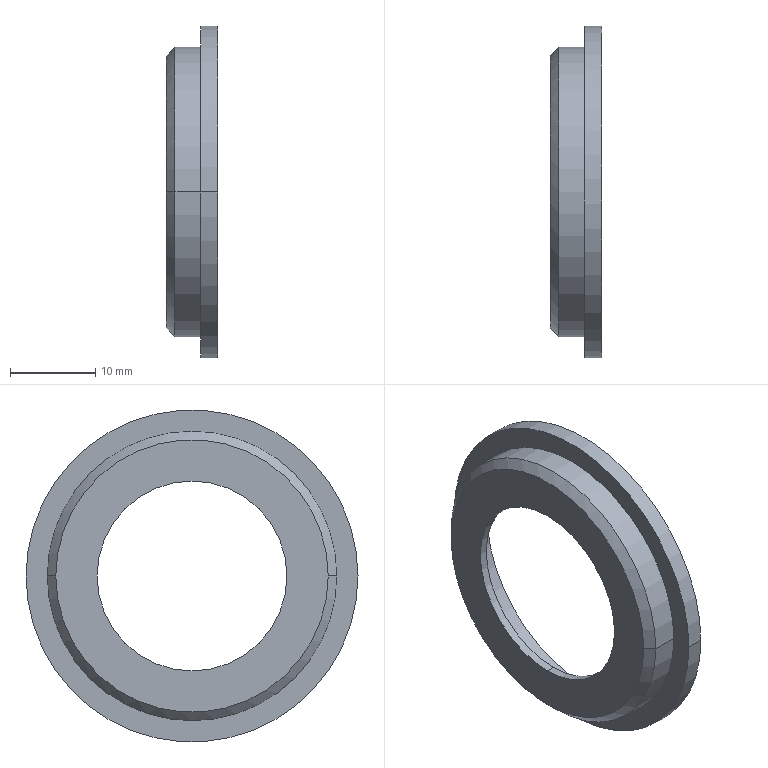Part | STEP file | Adjusting plate SGN-4-13 (19.5) | 1 solid | 15 faces | box 6 x 39 x 39 mm | volume 1841 mm3 | cylinder 8 | cone 4 | plane 3 | commonest cylinder face diameters 22.3 x2 32 x2 34 x2 39 x2
STEP:
#1=CARTESIAN_POINT('',(0.,0.,0.));
#2=DIRECTION('',(0.,0.,1.));
#3=DIRECTION('',(1.,0.,0.));
#4=AXIS2_PLACEMENT_3D('',#1,#2,#3);
#5=CARTESIAN_POINT('',(-6.,-16.,0.));
#6=VERTEX_POINT('',#5);
#7=CARTESIAN_POINT('',(-6.,16.,0.));
#8=VERTEX_POINT('',#7);
#9=CARTESIAN_POINT('',(-6.,0.,0.));
#10=DIRECTION('',(-1.,0.,0.));
#11=DIRECTION('',(0.,-1.,0.));
#12=AXIS2_PLACEMENT_3D('',#9,#10,#11);
#13=CIRCLE('',#12,16.);
#14=CARTESIAN_POINT('',(-5.,0.,0.));
#15=DIRECTION('',(1.,0.,0.));
#16=DIRECTION('',(0.,1.,0.));
#17=AXIS2_PLACEMENT_3D('',#14,#15,#16);
#18=CONICAL_SURFACE('',#17,17.,0.7854);
#19=CARTESIAN_POINT('',(3.142,-1.));
#20=DIRECTION('',(-1.,0.));
#21=VECTOR('',#20,1.);
#22=LINE('',#19,#21);
#23=(GEOMETRIC_REPRESENTATION_CONTEXT(2)PARAMETRIC_REPRESENTATION_CONTEXT()REPRESENTATION_CONTEXT('',''));
#24=DEFINITIONAL_REPRESENTATION('',(#22),#23);
#25=PCURVE('',#18,#24);
#26=CARTESIAN_POINT('',(-6.,17.,0.));
#27=DIRECTION('',(-1.,0.,0.));
#28=DIRECTION('',(0.,-1.,0.));
#29=AXIS2_PLACEMENT_3D('',#26,#27,#28);
#30=PLANE('',#29);
#31=CARTESIAN_POINT('',(17.,0.));
#32=DIRECTION('',(1.,0.));
#33=AXIS2_PLACEMENT_2D('',#31,#32);
#34=CIRCLE('',#33,16.);
#35=(GEOMETRIC_REPRESENTATION_CONTEXT(2)PARAMETRIC_REPRESENTATION_CONTEXT()REPRESENTATION_CONTEXT('',''));
#36=DEFINITIONAL_REPRESENTATION('',(#34),#35);
#37=PCURVE('',#30,#36);
#38=SURFACE_CURVE('',#13,(#25,#37),.PCURVE_S1.);
#39=EDGE_CURVE('',#6,#8,#38,.T.);
#40=ORIENTED_EDGE('',*,*,#39,.F.);
#41=CARTESIAN_POINT('',(-5.,-17.,0.));
#42=VERTEX_POINT('',#41);
#43=CARTESIAN_POINT('',(-5.,-17.,0.));
#44=DIRECTION('',(0.7071,-0.7071,0.));
#45=VECTOR('',#44,1.);
#46=LINE('',#43,#45);
#47=CARTESIAN_POINT('',(3.142,0.));
#48=DIRECTION('',(0.,1.));
#49=VECTOR('',#48,1.);
#50=LINE('',#47,#49);
#51=(GEOMETRIC_REPRESENTATION_CONTEXT(2)PARAMETRIC_REPRESENTATION_CONTEXT()REPRESENTATION_CONTEXT('',''));
#52=DEFINITIONAL_REPRESENTATION('',(#50),#51);
#53=PCURVE('',#18,#52);
#54=CARTESIAN_POINT('',(-5.,0.,0.));
#55=DIRECTION('',(1.,0.,0.));
#56=DIRECTION('',(0.,1.,0.));
#57=AXIS2_PLACEMENT_3D('',#54,#55,#56);
#58=CONICAL_SURFACE('',#57,17.,0.7854);
#59=CARTESIAN_POINT('',(3.142,0.));
#60=DIRECTION('',(0.,1.));
#61=VECTOR('',#60,1.);
#62=LINE('',#59,#61);
#63=(GEOMETRIC_REPRESENTATION_CONTEXT(2)PARAMETRIC_REPRESENTATION_CONTEXT()REPRESENTATION_CONTEXT('',''));
#64=DEFINITIONAL_REPRESENTATION('',(#62),#63);
#65=PCURVE('',#58,#64);
#66=SURFACE_CURVE('',#46,(#53,#65),.PCURVE_S1.);
#67=EDGE_CURVE('',#6,#42,#66,.T.);
#68=ORIENTED_EDGE('',*,*,#67,.T.);
#69=CARTESIAN_POINT('',(-5.,17.,0.));
#70=VERTEX_POINT('',#69);
#71=CARTESIAN_POINT('',(-5.,0.,0.));
#72=DIRECTION('',(1.,0.,0.));
#73=DIRECTION('',(0.,-1.,0.));
#74=AXIS2_PLACEMENT_3D('',#71,#72,#73);
#75=CIRCLE('',#74,17.);
#76=CARTESIAN_POINT('',(-3.142,0.));
#77=DIRECTION('',(1.,0.));
#78=VECTOR('',#77,1.);
#79=LINE('',#76,#78);
#80=(GEOMETRIC_REPRESENTATION_CONTEXT(2)PARAMETRIC_REPRESENTATION_CONTEXT()REPRESENTATION_CONTEXT('',''));
#81=DEFINITIONAL_REPRESENTATION('',(#79),#80);
#82=PCURVE('',#18,#81);
#83=CARTESIAN_POINT('',(0.,0.,0.));
#84=DIRECTION('',(1.,0.,0.));
#85=DIRECTION('',(0.,1.,0.));
#86=AXIS2_PLACEMENT_3D('',#83,#84,#85);
#87=CYLINDRICAL_SURFACE('',#86,17.);
#88=CARTESIAN_POINT('',(-3.142,-5.));
#89=DIRECTION('',(1.,0.));
#90=VECTOR('',#89,1.);
#91=LINE('',#88,#90);
#92=(GEOMETRIC_REPRESENTATION_CONTEXT(2)PARAMETRIC_REPRESENTATION_CONTEXT()REPRESENTATION_CONTEXT('',''));
#93=DEFINITIONAL_REPRESENTATION('',(#91),#92);
#94=PCURVE('',#87,#93);
#95=SURFACE_CURVE('',#75,(#82,#94),.PCURVE_S1.);
#96=EDGE_CURVE('',#70,#42,#95,.T.);
#97=ORIENTED_EDGE('',*,*,#96,.F.);
#98=CARTESIAN_POINT('',(-5.,17.,0.));
#99=DIRECTION('',(0.7071,0.7071,0.));
#100=VECTOR('',#99,1.);
#101=LINE('',#98,#100);
#102=CARTESIAN_POINT('',(0.,0.));
#103=DIRECTION('',(0.,1.));
#104=VECTOR('',#103,1.);
#105=LINE('',#102,#104);
#106=(GEOMETRIC_REPRESENTATION_CONTEXT(2)PARAMETRIC_REPRESENTATION_CONTEXT()REPRESENTATION_CONTEXT('',''));
#107=DEFINITIONAL_REPRESENTATION('',(#105),#106);
#108=PCURVE('',#18,#107);
#109=CARTESIAN_POINT('',(6.283,0.));
#110=DIRECTION('',(0.,1.));
#111=VECTOR('',#110,1.);
#112=LINE('',#109,#111);
#113=(GEOMETRIC_REPRESENTATION_CONTEXT(2)PARAMETRIC_REPRESENTATION_CONTEXT()REPRESENTATION_CONTEXT('',''));
#114=DEFINITIONAL_REPRESENTATION('',(#112),#113);
#115=PCURVE('',#58,#114);
#116=SURFACE_CURVE('',#101,(#108,#115),.PCURVE_S1.);
#117=EDGE_CURVE('',#8,#70,#116,.T.);
#118=ORIENTED_EDGE('',*,*,#117,.F.);
#119=EDGE_LOOP('',(#40,#68,#97,#118));
#120=FACE_BOUND('',#119,.T.);
#121=ADVANCED_FACE('',(#120),#18,.T.);
#122=CARTESIAN_POINT('',(-3.7,0.,-16.));
#123=VERTEX_POINT('',#122);
#124=CARTESIAN_POINT('',(0.,0.,-16.));
#125=VERTEX_POINT('',#124);
#126=CARTESIAN_POINT('',(0.,0.,-16.));
#127=DIRECTION('',(1.,0.,0.));
#128=VECTOR('',#127,1.);
#129=LINE('',#126,#128);
#130=CARTESIAN_POINT('',(0.,0.,0.));
#131=DIRECTION('',(1.,0.,0.));
#132=DIRECTION('',(0.,0.,-1.));
#133=AXIS2_PLACEMENT_3D('',#130,#131,#132);
#134=CYLINDRICAL_SURFACE('',#133,16.);
#135=CARTESIAN_POINT('',(6.283,0.));
#136=DIRECTION('',(0.,1.));
#137=VECTOR('',#136,1.);
#138=LINE('',#135,#137);
#139=(GEOMETRIC_REPRESENTATION_CONTEXT(2)PARAMETRIC_REPRESENTATION_CONTEXT()REPRESENTATION_CONTEXT('',''));
#140=DEFINITIONAL_REPRESENTATION('',(#138),#139);
#141=PCURVE('',#134,#140);
#142=CARTESIAN_POINT('',(0.,0.,0.));
#143=DIRECTION('',(1.,0.,0.));
#144=DIRECTION('',(0.,0.,-1.));
#145=AXIS2_PLACEMENT_3D('',#142,#143,#144);
#146=CYLINDRICAL_SURFACE('',#145,16.);
#147=CARTESIAN_POINT('',(0.,0.));
#148=DIRECTION('',(0.,1.));
#149=VECTOR('',#148,1.);
#150=LINE('',#147,#149);
#151=(GEOMETRIC_REPRESENTATION_CONTEXT(2)PARAMETRIC_REPRESENTATION_CONTEXT()REPRESENTATION_CONTEXT('',''));
#152=DEFINITIONAL_REPRESENTATION('',(#150),#151);
#153=PCURVE('',#146,#152);
#154=SURFACE_CURVE('',#129,(#141,#153),.PCURVE_S1.);
#155=EDGE_CURVE('',#123,#125,#154,.T.);
#156=ORIENTED_EDGE('',*,*,#155,.T.);
#157=CARTESIAN_POINT('',(0.,0.,16.));
#158=VERTEX_POINT('',#157);
#159=CARTESIAN_POINT('',(0.,0.,0.));
#160=DIRECTION('',(1.,0.,0.));
#161=DIRECTION('',(0.,0.,-1.));
#162=AXIS2_PLACEMENT_3D('',#159,#160,#161);
#163=CIRCLE('',#162,16.);
#164=CARTESIAN_POINT('',(0.,0.));
#165=DIRECTION('',(1.,0.));
#166=VECTOR('',#165,1.);
#167=LINE('',#164,#166);
#168=(GEOMETRIC_REPRESENTATION_CONTEXT(2)PARAMETRIC_REPRESENTATION_CONTEXT()REPRESENTATION_CONTEXT('',''));
#169=DEFINITIONAL_REPRESENTATION('',(#167),#168);
#170=PCURVE('',#134,#169);
#171=CARTESIAN_POINT('',(0.,0.,0.));
#172=DIRECTION('',(1.,0.,0.));
#173=DIRECTION('',(0.,1.,0.));
#174=AXIS2_PLACEMENT_3D('',#171,#172,#173);
#175=PLANE('',#174);
#176=CARTESIAN_POINT('',(0.,0.));
#177=DIRECTION('',(0.,-1.));
#178=AXIS2_PLACEMENT_2D('',#176,#177);
#179=CIRCLE('',#178,16.);
#180=(GEOMETRIC_REPRESENTATION_CONTEXT(2)PARAMETRIC_REPRESENTATION_CONTEXT()REPRESENTATION_CONTEXT('',''));
#181=DEFINITIONAL_REPRESENTATION('',(#179),#180);
#182=PCURVE('',#175,#181);
#183=SURFACE_CURVE('',#163,(#170,#182),.PCURVE_S1.);
#184=EDGE_CURVE('',#158,#125,#183,.T.);
#185=ORIENTED_EDGE('',*,*,#184,.F.);
#186=CARTESIAN_POINT('',(-3.7,0.,16.));
#187=VERTEX_POINT('',#186);
#188=CARTESIAN_POINT('',(0.,0.,16.));
#189=DIRECTION('',(1.,0.,0.));
#190=VECTOR('',#189,1.);
#191=LINE('',#188,#190);
#192=CARTESIAN_POINT('',(3.142,0.));
#193=DIRECTION('',(0.,1.));
#194=VECTOR('',#193,1.);
#195=LINE('',#192,#194);
#196=(GEOMETRIC_REPRESENTATION_CONTEXT(2)PARAMETRIC_REPRESENTATION_CONTEXT()REPRESENTATION_CONTEXT('',''));
#197=DEFINITIONAL_REPRESENTATION('',(#195),#196);
#198=PCURVE('',#134,#197);
#199=CARTESIAN_POINT('',(3.142,0.));
#200=DIRECTION('',(0.,1.));
#201=VECTOR('',#200,1.);
#202=LINE('',#199,#201);
#203=(GEOMETRIC_REPRESENTATION_CONTEXT(2)PARAMETRIC_REPRESENTATION_CONTEXT()REPRESENTATION_CONTEXT('',''));
#204=DEFINITIONAL_REPRESENTATION('',(#202),#203);
#205=PCURVE('',#146,#204);
#206=SURFACE_CURVE('',#191,(#198,#205),.PCURVE_S1.);
#207=EDGE_CURVE('',#187,#158,#206,.T.);
#208=ORIENTED_EDGE('',*,*,#207,.F.);
#209=CARTESIAN_POINT('',(-3.7,0.,0.));
#210=DIRECTION('',(1.,0.,0.));
#211=DIRECTION('',(0.,0.,-1.));
#212=AXIS2_PLACEMENT_3D('',#209,#210,#211);
#213=CIRCLE('',#212,16.);
#214=CARTESIAN_POINT('',(0.,-3.7));
#215=DIRECTION('',(1.,0.));
#216=VECTOR('',#215,1.);
#217=LINE('',#214,#216);
#218=(GEOMETRIC_REPRESENTATION_CONTEXT(2)PARAMETRIC_REPRESENTATION_CONTEXT()REPRESENTATION_CONTEXT('',''));
#219=DEFINITIONAL_REPRESENTATION('',(#217),#218);
#220=PCURVE('',#134,#219);
#221=CARTESIAN_POINT('',(-3.7,0.,0.));
#222=DIRECTION('',(1.,0.,0.));
#223=DIRECTION('',(0.,0.,-1.));
#224=AXIS2_PLACEMENT_3D('',#221,#222,#223);
#225=CONICAL_SURFACE('',#224,16.,1.309);
#226=CARTESIAN_POINT('',(0.,0.));
#227=DIRECTION('',(1.,0.));
#228=VECTOR('',#227,1.);
#229=LINE('',#226,#228);
#230=(GEOMETRIC_REPRESENTATION_CONTEXT(2)PARAMETRIC_REPRESENTATION_CONTEXT()REPRESENTATION_CONTEXT('',''));
#231=DEFINITIONAL_REPRESENTATION('',(#229),#230);
#232=PCURVE('',#225,#231);
#233=SURFACE_CURVE('',#213,(#220,#232),.PCURVE_S1.);
#234=EDGE_CURVE('',#187,#123,#233,.T.);
#235=ORIENTED_EDGE('',*,*,#234,.T.);
#236=EDGE_LOOP('',(#156,#185,#208,#235));
#237=FACE_BOUND('',#236,.F.);
#238=ADVANCED_FACE('',(#237),#134,.F.);
#239=CARTESIAN_POINT('',(-5.,0.,-11.15));
#240=VERTEX_POINT('',#239);
#241=CARTESIAN_POINT('',(-3.7,0.,-16.));
#242=DIRECTION('',(0.2588,0.,-0.9659));
#243=VECTOR('',#242,1.);
#244=LINE('',#241,#243);
#245=CARTESIAN_POINT('',(6.283,0.));
#246=DIRECTION('',(0.,1.));
#247=VECTOR('',#246,1.);
#248=LINE('',#245,#247);
#249=(GEOMETRIC_REPRESENTATION_CONTEXT(2)PARAMETRIC_REPRESENTATION_CONTEXT()REPRESENTATION_CONTEXT('',''));
#250=DEFINITIONAL_REPRESENTATION('',(#248),#249);
#251=PCURVE('',#225,#250);
#252=CARTESIAN_POINT('',(-3.7,0.,0.));
#253=DIRECTION('',(1.,0.,0.));
#254=DIRECTION('',(0.,0.,-1.));
#255=AXIS2_PLACEMENT_3D('',#252,#253,#254);
#256=CONICAL_SURFACE('',#255,16.,1.309);
#257=CARTESIAN_POINT('',(0.,0.));
#258=DIRECTION('',(0.,1.));
#259=VECTOR('',#258,1.);
#260=LINE('',#257,#259);
#261=(GEOMETRIC_REPRESENTATION_CONTEXT(2)PARAMETRIC_REPRESENTATION_CONTEXT()REPRESENTATION_CONTEXT('',''));
#262=DEFINITIONAL_REPRESENTATION('',(#260),#261);
#263=PCURVE('',#256,#262);
#264=SURFACE_CURVE('',#244,(#251,#263),.PCURVE_S1.);
#265=EDGE_CURVE('',#240,#123,#264,.T.);
#266=ORIENTED_EDGE('',*,*,#265,.T.);
#267=ORIENTED_EDGE('',*,*,#234,.F.);
#268=CARTESIAN_POINT('',(-5.,0.,11.15));
#269=VERTEX_POINT('',#268);
#270=CARTESIAN_POINT('',(-3.7,0.,16.));
#271=DIRECTION('',(0.2588,0.,0.9659));
#272=VECTOR('',#271,1.);
#273=LINE('',#270,#272);
#274=CARTESIAN_POINT('',(3.142,0.));
#275=DIRECTION('',(0.,1.));
#276=VECTOR('',#275,1.);
#277=LINE('',#274,#276);
#278=(GEOMETRIC_REPRESENTATION_CONTEXT(2)PARAMETRIC_REPRESENTATION_CONTEXT()REPRESENTATION_CONTEXT('',''));
#279=DEFINITIONAL_REPRESENTATION('',(#277),#278);
#280=PCURVE('',#225,#279);
#281=CARTESIAN_POINT('',(3.142,0.));
#282=DIRECTION('',(0.,1.));
#283=VECTOR('',#282,1.);
#284=LINE('',#281,#283);
#285=(GEOMETRIC_REPRESENTATION_CONTEXT(2)PARAMETRIC_REPRESENTATION_CONTEXT()REPRESENTATION_CONTEXT('',''));
#286=DEFINITIONAL_REPRESENTATION('',(#284),#285);
#287=PCURVE('',#256,#286);
#288=SURFACE_CURVE('',#273,(#280,#287),.PCURVE_S1.);
#289=EDGE_CURVE('',#269,#187,#288,.T.);
#290=ORIENTED_EDGE('',*,*,#289,.F.);
#291=CARTESIAN_POINT('',(-5.,0.,0.));
#292=DIRECTION('',(1.,0.,0.));
#293=DIRECTION('',(0.,0.,-1.));
#294=AXIS2_PLACEMENT_3D('',#291,#292,#293);
#295=CIRCLE('',#294,11.15);
#296=CARTESIAN_POINT('',(0.,-1.3));
#297=DIRECTION('',(1.,0.));
#298=VECTOR('',#297,1.);
#299=LINE('',#296,#298);
#300=(GEOMETRIC_REPRESENTATION_CONTEXT(2)PARAMETRIC_REPRESENTATION_CONTEXT()REPRESENTATION_CONTEXT('',''));
#301=DEFINITIONAL_REPRESENTATION('',(#299),#300);
#302=PCURVE('',#225,#301);
#303=CARTESIAN_POINT('',(-10.,0.,0.));
#304=DIRECTION('',(1.,0.,0.));
#305=DIRECTION('',(0.,0.,-1.));
#306=AXIS2_PLACEMENT_3D('',#303,#304,#305);
#307=CYLINDRICAL_SURFACE('',#306,11.15);
#308=CARTESIAN_POINT('',(0.,5.));
#309=DIRECTION('',(1.,0.));
#310=VECTOR('',#309,1.);
#311=LINE('',#308,#310);
#312=(GEOMETRIC_REPRESENTATION_CONTEXT(2)PARAMETRIC_REPRESENTATION_CONTEXT()REPRESENTATION_CONTEXT('',''));
#313=DEFINITIONAL_REPRESENTATION('',(#311),#312);
#314=PCURVE('',#307,#313);
#315=SURFACE_CURVE('',#295,(#302,#314),.PCURVE_S1.);
#316=EDGE_CURVE('',#269,#240,#315,.T.);
#317=ORIENTED_EDGE('',*,*,#316,.T.);
#318=EDGE_LOOP('',(#266,#267,#290,#317));
#319=FACE_BOUND('',#318,.F.);
#320=ADVANCED_FACE('',(#319),#225,.F.);
#321=CARTESIAN_POINT('',(-6.,0.,-11.15));
#322=VERTEX_POINT('',#321);
#323=CARTESIAN_POINT('',(-10.,0.,-11.15));
#324=DIRECTION('',(1.,0.,0.));
#325=VECTOR('',#324,1.);
#326=LINE('',#323,#325);
#327=CARTESIAN_POINT('',(6.283,0.));
#328=DIRECTION('',(0.,1.));
#329=VECTOR('',#328,1.);
#330=LINE('',#327,#329);
#331=(GEOMETRIC_REPRESENTATION_CONTEXT(2)PARAMETRIC_REPRESENTATION_CONTEXT()REPRESENTATION_CONTEXT('',''));
#332=DEFINITIONAL_REPRESENTATION('',(#330),#331);
#333=PCURVE('',#307,#332);
#334=CARTESIAN_POINT('',(-10.,0.,0.));
#335=DIRECTION('',(1.,0.,0.));
#336=DIRECTION('',(0.,0.,-1.));
#337=AXIS2_PLACEMENT_3D('',#334,#335,#336);
#338=CYLINDRICAL_SURFACE('',#337,11.15);
#339=CARTESIAN_POINT('',(0.,0.));
#340=DIRECTION('',(0.,1.));
#341=VECTOR('',#340,1.);
#342=LINE('',#339,#341);
#343=(GEOMETRIC_REPRESENTATION_CONTEXT(2)PARAMETRIC_REPRESENTATION_CONTEXT()REPRESENTATION_CONTEXT('',''));
#344=DEFINITIONAL_REPRESENTATION('',(#342),#343);
#345=PCURVE('',#338,#344);
#346=SURFACE_CURVE('',#326,(#333,#345),.PCURVE_S1.);
#347=EDGE_CURVE('',#322,#240,#346,.T.);
#348=ORIENTED_EDGE('',*,*,#347,.T.);
#349=ORIENTED_EDGE('',*,*,#316,.F.);
#350=CARTESIAN_POINT('',(-6.,0.,11.15));
#351=VERTEX_POINT('',#350);
#352=CARTESIAN_POINT('',(-10.,0.,11.15));
#353=DIRECTION('',(1.,0.,0.));
#354=VECTOR('',#353,1.);
#355=LINE('',#352,#354);
#356=CARTESIAN_POINT('',(3.142,0.));
#357=DIRECTION('',(0.,1.));
#358=VECTOR('',#357,1.);
#359=LINE('',#356,#358);
#360=(GEOMETRIC_REPRESENTATION_CONTEXT(2)PARAMETRIC_REPRESENTATION_CONTEXT()REPRESENTATION_CONTEXT('',''));
#361=DEFINITIONAL_REPRESENTATION('',(#359),#360);
#362=PCURVE('',#307,#361);
#363=CARTESIAN_POINT('',(3.142,0.));
#364=DIRECTION('',(0.,1.));
#365=VECTOR('',#364,1.);
#366=LINE('',#363,#365);
#367=(GEOMETRIC_REPRESENTATION_CONTEXT(2)PARAMETRIC_REPRESENTATION_CONTEXT()REPRESENTATION_CONTEXT('',''));
#368=DEFINITIONAL_REPRESENTATION('',(#366),#367);
#369=PCURVE('',#338,#368);
#370=SURFACE_CURVE('',#355,(#362,#369),.PCURVE_S1.);
#371=EDGE_CURVE('',#351,#269,#370,.T.);
#372=ORIENTED_EDGE('',*,*,#371,.F.);
#373=CARTESIAN_POINT('',(-6.,0.,0.));
#374=DIRECTION('',(-1.,0.,0.));
#375=DIRECTION('',(0.,-1.,0.));
#376=AXIS2_PLACEMENT_3D('',#373,#374,#375);
#377=CIRCLE('',#376,11.15);
#378=CARTESIAN_POINT('',(10.996,4.));
#379=DIRECTION('',(-1.,0.));
#380=VECTOR('',#379,1.);
#381=LINE('',#378,#380);
#382=(GEOMETRIC_REPRESENTATION_CONTEXT(2)PARAMETRIC_REPRESENTATION_CONTEXT()REPRESENTATION_CONTEXT('',''));
#383=DEFINITIONAL_REPRESENTATION('',(#381),#382);
#384=PCURVE('',#307,#383);
#385=CARTESIAN_POINT('',(17.,0.));
#386=DIRECTION('',(1.,0.));
#387=AXIS2_PLACEMENT_2D('',#385,#386);
#388=CIRCLE('',#387,11.15);
#389=(GEOMETRIC_REPRESENTATION_CONTEXT(2)PARAMETRIC_REPRESENTATION_CONTEXT()REPRESENTATION_CONTEXT('',''));
#390=DEFINITIONAL_REPRESENTATION('',(#388),#389);
#391=PCURVE('',#30,#390);
#392=SURFACE_CURVE('',#377,(#384,#391),.PCURVE_S1.);
#393=EDGE_CURVE('',#322,#351,#392,.T.);
#394=ORIENTED_EDGE('',*,*,#393,.F.);
#395=EDGE_LOOP('',(#348,#349,#372,#394));
#396=FACE_BOUND('',#395,.F.);
#397=ADVANCED_FACE('',(#396),#307,.F.);
#398=ORIENTED_EDGE('',*,*,#96,.T.);
#399=CARTESIAN_POINT('',(-2.,-17.,0.));
#400=VERTEX_POINT('',#399);
#401=CARTESIAN_POINT('',(0.,-17.,0.));
#402=DIRECTION('',(1.,0.,0.));
#403=VECTOR('',#402,1.);
#404=LINE('',#401,#403);
#405=CARTESIAN_POINT('',(3.142,0.));
#406=DIRECTION('',(0.,1.));
#407=VECTOR('',#406,1.);
#408=LINE('',#405,#407);
#409=(GEOMETRIC_REPRESENTATION_CONTEXT(2)PARAMETRIC_REPRESENTATION_CONTEXT()REPRESENTATION_CONTEXT('',''));
#410=DEFINITIONAL_REPRESENTATION('',(#408),#409);
#411=PCURVE('',#87,#410);
#412=CARTESIAN_POINT('',(0.,0.,0.));
#413=DIRECTION('',(1.,0.,0.));
#414=DIRECTION('',(0.,1.,0.));
#415=AXIS2_PLACEMENT_3D('',#412,#413,#414);
#416=CYLINDRICAL_SURFACE('',#415,17.);
#417=CARTESIAN_POINT('',(3.142,0.));
#418=DIRECTION('',(0.,1.));
#419=VECTOR('',#418,1.);
#420=LINE('',#417,#419);
#421=(GEOMETRIC_REPRESENTATION_CONTEXT(2)PARAMETRIC_REPRESENTATION_CONTEXT()REPRESENTATION_CONTEXT('',''));
#422=DEFINITIONAL_REPRESENTATION('',(#420),#421);
#423=PCURVE('',#416,#422);
#424=SURFACE_CURVE('',#404,(#411,#423),.PCURVE_S1.);
#425=EDGE_CURVE('',#42,#400,#424,.T.);
#426=ORIENTED_EDGE('',*,*,#425,.T.);
#427=CARTESIAN_POINT('',(-2.,17.,0.));
#428=VERTEX_POINT('',#427);
#429=CARTESIAN_POINT('',(-2.,0.,0.));
#430=DIRECTION('',(1.,0.,0.));
#431=DIRECTION('',(0.,1.,0.));
#432=AXIS2_PLACEMENT_3D('',#429,#430,#431);
#433=CIRCLE('',#432,17.);
#434=CARTESIAN_POINT('',(0.,-2.));
#435=DIRECTION('',(1.,0.));
#436=VECTOR('',#435,1.);
#437=LINE('',#434,#436);
#438=(GEOMETRIC_REPRESENTATION_CONTEXT(2)PARAMETRIC_REPRESENTATION_CONTEXT()REPRESENTATION_CONTEXT('',''));
#439=DEFINITIONAL_REPRESENTATION('',(#437),#438);
#440=PCURVE('',#87,#439);
#441=CARTESIAN_POINT('',(-2.,19.5,0.));
#442=DIRECTION('',(-1.,0.,0.));
#443=DIRECTION('',(0.,-1.,0.));
#444=AXIS2_PLACEMENT_3D('',#441,#442,#443);
#445=PLANE('',#444);
#446=CARTESIAN_POINT('',(2.5,0.));
#447=CARTESIAN_POINT('',(2.5,29.445));
#448=CARTESIAN_POINT('',(28.,14.722));
#449=CARTESIAN_POINT('',(53.5,0.));
#450=CARTESIAN_POINT('',(28.,-14.722));
#451=CARTESIAN_POINT('',(2.5,-29.445));
#452=CARTESIAN_POINT('',(2.5,0.));
#453=(BOUNDED_CURVE()B_SPLINE_CURVE(2,(#446,#447,#448,#449,#450,#451,#452),.UNSPECIFIED.,.T.,.F.)B_SPLINE_CURVE_WITH_KNOTS((1,2,2,2,2,1),(-2.094,0.,2.094,4.189,6.283,8.378),.UNSPECIFIED.)CURVE()GEOMETRIC_REPRESENTATION_ITEM()RATIONAL_B_SPLINE_CURVE((1.,0.5,1.,0.5,1.,0.5,1.))REPRESENTATION_ITEM(''));
#454=(GEOMETRIC_REPRESENTATION_CONTEXT(2)PARAMETRIC_REPRESENTATION_CONTEXT()REPRESENTATION_CONTEXT('',''));
#455=DEFINITIONAL_REPRESENTATION('',(#453),#454);
#456=PCURVE('',#445,#455);
#457=SURFACE_CURVE('',#433,(#440,#456),.PCURVE_S1.);
#458=EDGE_CURVE('',#428,#400,#457,.T.);
#459=ORIENTED_EDGE('',*,*,#458,.F.);
#460=CARTESIAN_POINT('',(0.,17.,0.));
#461=DIRECTION('',(1.,0.,0.));
#462=VECTOR('',#461,1.);
#463=LINE('',#460,#462);
#464=CARTESIAN_POINT('',(0.,0.));
#465=DIRECTION('',(0.,1.));
#466=VECTOR('',#465,1.);
#467=LINE('',#464,#466);
#468=(GEOMETRIC_REPRESENTATION_CONTEXT(2)PARAMETRIC_REPRESENTATION_CONTEXT()REPRESENTATION_CONTEXT('',''));
#469=DEFINITIONAL_REPRESENTATION('',(#467),#468);
#470=PCURVE('',#87,#469);
#471=CARTESIAN_POINT('',(6.283,0.));
#472=DIRECTION('',(0.,1.));
#473=VECTOR('',#472,1.);
#474=LINE('',#471,#473);
#475=(GEOMETRIC_REPRESENTATION_CONTEXT(2)PARAMETRIC_REPRESENTATION_CONTEXT()REPRESENTATION_CONTEXT('',''));
#476=DEFINITIONAL_REPRESENTATION('',(#474),#475);
#477=PCURVE('',#416,#476);
#478=SURFACE_CURVE('',#463,(#470,#477),.PCURVE_S1.);
#479=EDGE_CURVE('',#70,#428,#478,.T.);
#480=ORIENTED_EDGE('',*,*,#479,.F.);
#481=EDGE_LOOP('',(#398,#426,#459,#480));
#482=FACE_BOUND('',#481,.T.);
#483=ADVANCED_FACE('',(#482),#87,.T.);
#484=CARTESIAN_POINT('',(-2.,19.5,0.));
#485=VERTEX_POINT('',#484);
#486=CARTESIAN_POINT('',(-2.,-19.5,0.));
#487=VERTEX_POINT('',#486);
#488=CARTESIAN_POINT('',(-2.,0.,0.));
#489=DIRECTION('',(1.,0.,0.));
#490=DIRECTION('',(0.,1.,0.));
#491=AXIS2_PLACEMENT_3D('',#488,#489,#490);
#492=CIRCLE('',#491,19.5);
#493=CARTESIAN_POINT('',(0.,0.,0.));
#494=DIRECTION('',(1.,0.,0.));
#495=DIRECTION('',(0.,1.,0.));
#496=AXIS2_PLACEMENT_3D('',#493,#494,#495);
#497=CYLINDRICAL_SURFACE('',#496,19.5);
#498=CARTESIAN_POINT('',(0.,-2.));
#499=DIRECTION('',(1.,0.));
#500=VECTOR('',#499,1.);
#501=LINE('',#498,#500);
#502=(GEOMETRIC_REPRESENTATION_CONTEXT(2)PARAMETRIC_REPRESENTATION_CONTEXT()REPRESENTATION_CONTEXT('',''));
#503=DEFINITIONAL_REPRESENTATION('',(#501),#502);
#504=PCURVE('',#497,#503);
#505=CARTESIAN_POINT('',(0.,0.));
#506=CARTESIAN_POINT('',(0.,33.775));
#507=CARTESIAN_POINT('',(29.25,16.887));
#508=CARTESIAN_POINT('',(58.5,0.));
#509=CARTESIAN_POINT('',(29.25,-16.887));
#510=CARTESIAN_POINT('',(0.,-33.775));
#511=CARTESIAN_POINT('',(0.,0.));
#512=(BOUNDED_CURVE()B_SPLINE_CURVE(2,(#505,#506,#507,#508,#509,#510,#511),.UNSPECIFIED.,.T.,.F.)B_SPLINE_CURVE_WITH_KNOTS((1,2,2,2,2,1),(-2.094,0.,2.094,4.189,6.283,8.378),.UNSPECIFIED.)CURVE()GEOMETRIC_REPRESENTATION_ITEM()RATIONAL_B_SPLINE_CURVE((1.,0.5,1.,0.5,1.,0.5,1.))REPRESENTATION_ITEM(''));
#513=(GEOMETRIC_REPRESENTATION_CONTEXT(2)PARAMETRIC_REPRESENTATION_CONTEXT()REPRESENTATION_CONTEXT('',''));
#514=DEFINITIONAL_REPRESENTATION('',(#512),#513);
#515=PCURVE('',#445,#514);
#516=SURFACE_CURVE('',#492,(#504,#515),.PCURVE_S1.);
#517=EDGE_CURVE('',#485,#487,#516,.T.);
#518=ORIENTED_EDGE('',*,*,#517,.T.);
#519=CARTESIAN_POINT('',(0.,-19.5,0.));
#520=VERTEX_POINT('',#519);
#521=CARTESIAN_POINT('',(0.,-19.5,0.));
#522=DIRECTION('',(1.,0.,0.));
#523=VECTOR('',#522,1.);
#524=LINE('',#521,#523);
#525=CARTESIAN_POINT('',(3.142,0.));
#526=DIRECTION('',(0.,1.));
#527=VECTOR('',#526,1.);
#528=LINE('',#525,#527);
#529=(GEOMETRIC_REPRESENTATION_CONTEXT(2)PARAMETRIC_REPRESENTATION_CONTEXT()REPRESENTATION_CONTEXT('',''));
#530=DEFINITIONAL_REPRESENTATION('',(#528),#529);
#531=PCURVE('',#497,#530);
#532=CARTESIAN_POINT('',(0.,0.,0.));
#533=DIRECTION('',(1.,0.,0.));
#534=DIRECTION('',(0.,1.,0.));
#535=AXIS2_PLACEMENT_3D('',#532,#533,#534);
#536=CYLINDRICAL_SURFACE('',#535,19.5);
#537=CARTESIAN_POINT('',(3.142,0.));
#538=DIRECTION('',(0.,1.));
#539=VECTOR('',#538,1.);
#540=LINE('',#537,#539);
#541=(GEOMETRIC_REPRESENTATION_CONTEXT(2)PARAMETRIC_REPRESENTATION_CONTEXT()REPRESENTATION_CONTEXT('',''));
#542=DEFINITIONAL_REPRESENTATION('',(#540),#541);
#543=PCURVE('',#536,#542);
#544=SURFACE_CURVE('',#524,(#531,#543),.PCURVE_S1.);
#545=EDGE_CURVE('',#487,#520,#544,.T.);
#546=ORIENTED_EDGE('',*,*,#545,.T.);
#547=CARTESIAN_POINT('',(0.,19.5,0.));
#548=VERTEX_POINT('',#547);
#549=CARTESIAN_POINT('',(0.,0.,0.));
#550=DIRECTION('',(1.,0.,0.));
#551=DIRECTION('',(0.,1.,0.));
#552=AXIS2_PLACEMENT_3D('',#549,#550,#551);
#553=CIRCLE('',#552,19.5);
#554=CARTESIAN_POINT('',(0.,0.));
#555=DIRECTION('',(1.,0.));
#556=VECTOR('',#555,1.);
#557=LINE('',#554,#556);
#558=(GEOMETRIC_REPRESENTATION_CONTEXT(2)PARAMETRIC_REPRESENTATION_CONTEXT()REPRESENTATION_CONTEXT('',''));
#559=DEFINITIONAL_REPRESENTATION('',(#557),#558);
#560=PCURVE('',#497,#559);
#561=CARTESIAN_POINT('',(0.,0.));
#562=DIRECTION('',(1.,0.));
#563=AXIS2_PLACEMENT_2D('',#561,#562);
#564=CIRCLE('',#563,19.5);
#565=(GEOMETRIC_REPRESENTATION_CONTEXT(2)PARAMETRIC_REPRESENTATION_CONTEXT()REPRESENTATION_CONTEXT('',''));
#566=DEFINITIONAL_REPRESENTATION('',(#564),#565);
#567=PCURVE('',#175,#566);
#568=SURFACE_CURVE('',#553,(#560,#567),.PCURVE_S1.);
#569=EDGE_CURVE('',#548,#520,#568,.T.);
#570=ORIENTED_EDGE('',*,*,#569,.F.);
#571=CARTESIAN_POINT('',(0.,19.5,0.));
#572=DIRECTION('',(1.,0.,0.));
#573=VECTOR('',#572,1.);
#574=LINE('',#571,#573);
#575=CARTESIAN_POINT('',(0.,0.));
#576=DIRECTION('',(0.,1.));
#577=VECTOR('',#576,1.);
#578=LINE('',#575,#577);
#579=(GEOMETRIC_REPRESENTATION_CONTEXT(2)PARAMETRIC_REPRESENTATION_CONTEXT()REPRESENTATION_CONTEXT('',''));
#580=DEFINITIONAL_REPRESENTATION('',(#578),#579);
#581=PCURVE('',#497,#580);
#582=CARTESIAN_POINT('',(6.283,0.));
#583=DIRECTION('',(0.,1.));
#584=VECTOR('',#583,1.);
#585=LINE('',#582,#584);
#586=(GEOMETRIC_REPRESENTATION_CONTEXT(2)PARAMETRIC_REPRESENTATION_CONTEXT()REPRESENTATION_CONTEXT('',''));
#587=DEFINITIONAL_REPRESENTATION('',(#585),#586);
#588=PCURVE('',#536,#587);
#589=SURFACE_CURVE('',#574,(#581,#588),.PCURVE_S1.);
#590=EDGE_CURVE('',#485,#548,#589,.T.);
#591=ORIENTED_EDGE('',*,*,#590,.F.);
#592=EDGE_LOOP('',(#518,#546,#570,#591));
#593=FACE_BOUND('',#592,.T.);
#594=ADVANCED_FACE('',(#593),#497,.T.);
#595=CARTESIAN_POINT('',(0.,0.,0.));
#596=DIRECTION('',(1.,0.,0.));
#597=DIRECTION('',(0.,0.,-1.));
#598=AXIS2_PLACEMENT_3D('',#595,#596,#597);
#599=CIRCLE('',#598,16.);
#600=CARTESIAN_POINT('',(0.,0.));
#601=DIRECTION('',(0.,-1.));
#602=AXIS2_PLACEMENT_2D('',#600,#601);
#603=CIRCLE('',#602,16.);
#604=(GEOMETRIC_REPRESENTATION_CONTEXT(2)PARAMETRIC_REPRESENTATION_CONTEXT()REPRESENTATION_CONTEXT('',''));
#605=DEFINITIONAL_REPRESENTATION('',(#603),#604);
#606=PCURVE('',#175,#605);
#607=CARTESIAN_POINT('',(0.,0.));
#608=DIRECTION('',(1.,0.));
#609=VECTOR('',#608,1.);
#610=LINE('',#607,#609);
#611=(GEOMETRIC_REPRESENTATION_CONTEXT(2)PARAMETRIC_REPRESENTATION_CONTEXT()REPRESENTATION_CONTEXT('',''));
#612=DEFINITIONAL_REPRESENTATION('',(#610),#611);
#613=PCURVE('',#146,#612);
#614=SURFACE_CURVE('',#599,(#606,#613),.PCURVE_S1.);
#615=EDGE_CURVE('',#125,#158,#614,.T.);
#616=ORIENTED_EDGE('',*,*,#615,.F.);
#617=ORIENTED_EDGE('',*,*,#184,.F.);
#618=EDGE_LOOP('',(#616,#617));
#619=FACE_BOUND('',#618,.T.);
#620=ORIENTED_EDGE('',*,*,#569,.T.);
#621=CARTESIAN_POINT('',(0.,0.,0.));
#622=DIRECTION('',(1.,0.,0.));
#623=DIRECTION('',(0.,1.,0.));
#624=AXIS2_PLACEMENT_3D('',#621,#622,#623);
#625=CIRCLE('',#624,19.5);
#626=CARTESIAN_POINT('',(0.,0.));
#627=DIRECTION('',(1.,0.));
#628=AXIS2_PLACEMENT_2D('',#626,#627);
#629=CIRCLE('',#628,19.5);
#630=(GEOMETRIC_REPRESENTATION_CONTEXT(2)PARAMETRIC_REPRESENTATION_CONTEXT()REPRESENTATION_CONTEXT('',''));
#631=DEFINITIONAL_REPRESENTATION('',(#629),#630);
#632=PCURVE('',#175,#631);
#633=CARTESIAN_POINT('',(0.,0.));
#634=DIRECTION('',(1.,0.));
#635=VECTOR('',#634,1.);
#636=LINE('',#633,#635);
#637=(GEOMETRIC_REPRESENTATION_CONTEXT(2)PARAMETRIC_REPRESENTATION_CONTEXT()REPRESENTATION_CONTEXT('',''));
#638=DEFINITIONAL_REPRESENTATION('',(#636),#637);
#639=PCURVE('',#536,#638);
#640=SURFACE_CURVE('',#625,(#632,#639),.PCURVE_S1.);
#641=EDGE_CURVE('',#520,#548,#640,.T.);
#642=ORIENTED_EDGE('',*,*,#641,.T.);
#643=EDGE_LOOP('',(#620,#642));
#644=FACE_BOUND('',#643,.T.);
#645=ADVANCED_FACE('',(#619,#644),#175,.T.);
#646=ORIENTED_EDGE('',*,*,#545,.F.);
#647=CARTESIAN_POINT('',(-2.,0.,0.));
#648=DIRECTION('',(1.,0.,0.));
#649=DIRECTION('',(0.,1.,0.));
#650=AXIS2_PLACEMENT_3D('',#647,#648,#649);
#651=CIRCLE('',#650,19.5);
#652=CARTESIAN_POINT('',(0.,-2.));
#653=DIRECTION('',(1.,0.));
#654=VECTOR('',#653,1.);
#655=LINE('',#652,#654);
#656=(GEOMETRIC_REPRESENTATION_CONTEXT(2)PARAMETRIC_REPRESENTATION_CONTEXT()REPRESENTATION_CONTEXT('',''));
#657=DEFINITIONAL_REPRESENTATION('',(#655),#656);
#658=PCURVE('',#536,#657);
#659=CARTESIAN_POINT('',(0.,0.));
#660=CARTESIAN_POINT('',(0.,33.775));
#661=CARTESIAN_POINT('',(29.25,16.887));
#662=CARTESIAN_POINT('',(58.5,0.));
#663=CARTESIAN_POINT('',(29.25,-16.887));
#664=CARTESIAN_POINT('',(0.,-33.775));
#665=CARTESIAN_POINT('',(0.,0.));
#666=(BOUNDED_CURVE()B_SPLINE_CURVE(2,(#659,#660,#661,#662,#663,#664,#665),.UNSPECIFIED.,.T.,.F.)B_SPLINE_CURVE_WITH_KNOTS((1,2,2,2,2,1),(-2.094,0.,2.094,4.189,6.283,8.378),.UNSPECIFIED.)CURVE()GEOMETRIC_REPRESENTATION_ITEM()RATIONAL_B_SPLINE_CURVE((1.,0.5,1.,0.5,1.,0.5,1.))REPRESENTATION_ITEM(''));
#667=(GEOMETRIC_REPRESENTATION_CONTEXT(2)PARAMETRIC_REPRESENTATION_CONTEXT()REPRESENTATION_CONTEXT('',''));
#668=DEFINITIONAL_REPRESENTATION('',(#666),#667);
#669=PCURVE('',#445,#668);
#670=SURFACE_CURVE('',#651,(#658,#669),.PCURVE_S1.);
#671=EDGE_CURVE('',#487,#485,#670,.T.);
#672=ORIENTED_EDGE('',*,*,#671,.T.);
#673=ORIENTED_EDGE('',*,*,#590,.T.);
#674=ORIENTED_EDGE('',*,*,#641,.F.);
#675=EDGE_LOOP('',(#646,#672,#673,#674));
#676=FACE_BOUND('',#675,.T.);
#677=ADVANCED_FACE('',(#676),#536,.T.);
#678=ORIENTED_EDGE('',*,*,#458,.T.);
#679=CARTESIAN_POINT('',(-2.,0.,0.));
#680=DIRECTION('',(1.,0.,0.));
#681=DIRECTION('',(0.,1.,0.));
#682=AXIS2_PLACEMENT_3D('',#679,#680,#681);
#683=CIRCLE('',#682,17.);
#684=CARTESIAN_POINT('',(2.5,0.));
#685=CARTESIAN_POINT('',(2.5,29.445));
#686=CARTESIAN_POINT('',(28.,14.722));
#687=CARTESIAN_POINT('',(53.5,0.));
#688=CARTESIAN_POINT('',(28.,-14.722));
#689=CARTESIAN_POINT('',(2.5,-29.445));
#690=CARTESIAN_POINT('',(2.5,0.));
#691=(BOUNDED_CURVE()B_SPLINE_CURVE(2,(#684,#685,#686,#687,#688,#689,#690),.UNSPECIFIED.,.T.,.F.)B_SPLINE_CURVE_WITH_KNOTS((1,2,2,2,2,1),(-2.094,0.,2.094,4.189,6.283,8.378),.UNSPECIFIED.)CURVE()GEOMETRIC_REPRESENTATION_ITEM()RATIONAL_B_SPLINE_CURVE((1.,0.5,1.,0.5,1.,0.5,1.))REPRESENTATION_ITEM(''));
#692=(GEOMETRIC_REPRESENTATION_CONTEXT(2)PARAMETRIC_REPRESENTATION_CONTEXT()REPRESENTATION_CONTEXT('',''));
#693=DEFINITIONAL_REPRESENTATION('',(#691),#692);
#694=PCURVE('',#445,#693);
#695=CARTESIAN_POINT('',(0.,-2.));
#696=DIRECTION('',(1.,0.));
#697=VECTOR('',#696,1.);
#698=LINE('',#695,#697);
#699=(GEOMETRIC_REPRESENTATION_CONTEXT(2)PARAMETRIC_REPRESENTATION_CONTEXT()REPRESENTATION_CONTEXT('',''));
#700=DEFINITIONAL_REPRESENTATION('',(#698),#699);
#701=PCURVE('',#416,#700);
#702=SURFACE_CURVE('',#683,(#694,#701),.PCURVE_S1.);
#703=EDGE_CURVE('',#400,#428,#702,.T.);
#704=ORIENTED_EDGE('',*,*,#703,.T.);
#705=EDGE_LOOP('',(#678,#704));
#706=FACE_BOUND('',#705,.T.);
#707=ORIENTED_EDGE('',*,*,#517,.F.);
#708=ORIENTED_EDGE('',*,*,#671,.F.);
#709=EDGE_LOOP('',(#707,#708));
#710=FACE_BOUND('',#709,.T.);
#711=ADVANCED_FACE('',(#706,#710),#445,.T.);
#712=ORIENTED_EDGE('',*,*,#425,.F.);
#713=CARTESIAN_POINT('',(-5.,0.,0.));
#714=DIRECTION('',(1.,0.,0.));
#715=DIRECTION('',(0.,-1.,0.));
#716=AXIS2_PLACEMENT_3D('',#713,#714,#715);
#717=CIRCLE('',#716,17.);
#718=CARTESIAN_POINT('',(3.142,-5.));
#719=DIRECTION('',(1.,0.));
#720=VECTOR('',#719,1.);
#721=LINE('',#718,#720);
#722=(GEOMETRIC_REPRESENTATION_CONTEXT(2)PARAMETRIC_REPRESENTATION_CONTEXT()REPRESENTATION_CONTEXT('',''));
#723=DEFINITIONAL_REPRESENTATION('',(#721),#722);
#724=PCURVE('',#416,#723);
#725=CARTESIAN_POINT('',(3.142,0.));
#726=DIRECTION('',(1.,0.));
#727=VECTOR('',#726,1.);
#728=LINE('',#725,#727);
#729=(GEOMETRIC_REPRESENTATION_CONTEXT(2)PARAMETRIC_REPRESENTATION_CONTEXT()REPRESENTATION_CONTEXT('',''));
#730=DEFINITIONAL_REPRESENTATION('',(#728),#729);
#731=PCURVE('',#58,#730);
#732=SURFACE_CURVE('',#717,(#724,#731),.PCURVE_S1.);
#733=EDGE_CURVE('',#42,#70,#732,.T.);
#734=ORIENTED_EDGE('',*,*,#733,.T.);
#735=ORIENTED_EDGE('',*,*,#479,.T.);
#736=ORIENTED_EDGE('',*,*,#703,.F.);
#737=EDGE_LOOP('',(#712,#734,#735,#736));
#738=FACE_BOUND('',#737,.T.);
#739=ADVANCED_FACE('',(#738),#416,.T.);
#740=CARTESIAN_POINT('',(-6.,0.,0.));
#741=DIRECTION('',(-1.,0.,0.));
#742=DIRECTION('',(0.,-1.,0.));
#743=AXIS2_PLACEMENT_3D('',#740,#741,#742);
#744=CIRCLE('',#743,16.);
#745=CARTESIAN_POINT('',(17.,0.));
#746=DIRECTION('',(1.,0.));
#747=AXIS2_PLACEMENT_2D('',#745,#746);
#748=CIRCLE('',#747,16.);
#749=(GEOMETRIC_REPRESENTATION_CONTEXT(2)PARAMETRIC_REPRESENTATION_CONTEXT()REPRESENTATION_CONTEXT('',''));
#750=DEFINITIONAL_REPRESENTATION('',(#748),#749);
#751=PCURVE('',#30,#750);
#752=CARTESIAN_POINT('',(9.425,-1.));
#753=DIRECTION('',(-1.,0.));
#754=VECTOR('',#753,1.);
#755=LINE('',#752,#754);
#756=(GEOMETRIC_REPRESENTATION_CONTEXT(2)PARAMETRIC_REPRESENTATION_CONTEXT()REPRESENTATION_CONTEXT('',''));
#757=DEFINITIONAL_REPRESENTATION('',(#755),#756);
#758=PCURVE('',#58,#757);
#759=SURFACE_CURVE('',#744,(#751,#758),.PCURVE_S1.);
#760=EDGE_CURVE('',#8,#6,#759,.T.);
#761=ORIENTED_EDGE('',*,*,#760,.T.);
#762=ORIENTED_EDGE('',*,*,#39,.T.);
#763=EDGE_LOOP('',(#761,#762));
#764=FACE_BOUND('',#763,.T.);
#765=ORIENTED_EDGE('',*,*,#393,.F.);
#766=CARTESIAN_POINT('',(-6.,0.,0.));
#767=DIRECTION('',(-1.,0.,0.));
#768=DIRECTION('',(0.,-1.,0.));
#769=AXIS2_PLACEMENT_3D('',#766,#767,#768);
#770=CIRCLE('',#769,11.15);
#771=CARTESIAN_POINT('',(17.,0.));
#772=DIRECTION('',(1.,0.));
#773=AXIS2_PLACEMENT_2D('',#771,#772);
#774=CIRCLE('',#773,11.15);
#775=(GEOMETRIC_REPRESENTATION_CONTEXT(2)PARAMETRIC_REPRESENTATION_CONTEXT()REPRESENTATION_CONTEXT('',''));
#776=DEFINITIONAL_REPRESENTATION('',(#774),#775);
#777=PCURVE('',#30,#776);
#778=CARTESIAN_POINT('',(4.712,4.));
#779=DIRECTION('',(-1.,0.));
#780=VECTOR('',#779,1.);
#781=LINE('',#778,#780);
#782=(GEOMETRIC_REPRESENTATION_CONTEXT(2)PARAMETRIC_REPRESENTATION_CONTEXT()REPRESENTATION_CONTEXT('',''));
#783=DEFINITIONAL_REPRESENTATION('',(#781),#782);
#784=PCURVE('',#338,#783);
#785=SURFACE_CURVE('',#770,(#777,#784),.PCURVE_S1.);
#786=EDGE_CURVE('',#351,#322,#785,.T.);
#787=ORIENTED_EDGE('',*,*,#786,.F.);
#788=EDGE_LOOP('',(#765,#787));
#789=FACE_BOUND('',#788,.T.);
#790=ADVANCED_FACE('',(#764,#789),#30,.T.);
#791=CARTESIAN_POINT('',(-5.,0.,0.));
#792=DIRECTION('',(1.,0.,0.));
#793=DIRECTION('',(0.,0.,-1.));
#794=AXIS2_PLACEMENT_3D('',#791,#792,#793);
#795=CIRCLE('',#794,11.15);
#796=CARTESIAN_POINT('',(0.,5.));
#797=DIRECTION('',(1.,0.));
#798=VECTOR('',#797,1.);
#799=LINE('',#796,#798);
#800=(GEOMETRIC_REPRESENTATION_CONTEXT(2)PARAMETRIC_REPRESENTATION_CONTEXT()REPRESENTATION_CONTEXT('',''));
#801=DEFINITIONAL_REPRESENTATION('',(#799),#800);
#802=PCURVE('',#338,#801);
#803=CARTESIAN_POINT('',(0.,-1.3));
#804=DIRECTION('',(1.,0.));
#805=VECTOR('',#804,1.);
#806=LINE('',#803,#805);
#807=(GEOMETRIC_REPRESENTATION_CONTEXT(2)PARAMETRIC_REPRESENTATION_CONTEXT()REPRESENTATION_CONTEXT('',''));
#808=DEFINITIONAL_REPRESENTATION('',(#806),#807);
#809=PCURVE('',#256,#808);
#810=SURFACE_CURVE('',#795,(#802,#809),.PCURVE_S1.);
#811=EDGE_CURVE('',#240,#269,#810,.T.);
#812=ORIENTED_EDGE('',*,*,#811,.F.);
#813=ORIENTED_EDGE('',*,*,#347,.F.);
#814=ORIENTED_EDGE('',*,*,#786,.F.);
#815=ORIENTED_EDGE('',*,*,#371,.T.);
#816=EDGE_LOOP('',(#812,#813,#814,#815));
#817=FACE_BOUND('',#816,.F.);
#818=ADVANCED_FACE('',(#817),#338,.F.);
#819=CARTESIAN_POINT('',(-3.7,0.,0.));
#820=DIRECTION('',(1.,0.,0.));
#821=DIRECTION('',(0.,0.,-1.));
#822=AXIS2_PLACEMENT_3D('',#819,#820,#821);
#823=CIRCLE('',#822,16.);
#824=CARTESIAN_POINT('',(0.,0.));
#825=DIRECTION('',(1.,0.));
#826=VECTOR('',#825,1.);
#827=LINE('',#824,#826);
#828=(GEOMETRIC_REPRESENTATION_CONTEXT(2)PARAMETRIC_REPRESENTATION_CONTEXT()REPRESENTATION_CONTEXT('',''));
#829=DEFINITIONAL_REPRESENTATION('',(#827),#828);
#830=PCURVE('',#256,#829);
#831=CARTESIAN_POINT('',(0.,-3.7));
#832=DIRECTION('',(1.,0.));
#833=VECTOR('',#832,1.);
#834=LINE('',#831,#833);
#835=(GEOMETRIC_REPRESENTATION_CONTEXT(2)PARAMETRIC_REPRESENTATION_CONTEXT()REPRESENTATION_CONTEXT('',''));
#836=DEFINITIONAL_REPRESENTATION('',(#834),#835);
#837=PCURVE('',#146,#836);
#838=SURFACE_CURVE('',#823,(#830,#837),.PCURVE_S1.);
#839=EDGE_CURVE('',#123,#187,#838,.T.);
#840=ORIENTED_EDGE('',*,*,#839,.F.);
#841=ORIENTED_EDGE('',*,*,#265,.F.);
#842=ORIENTED_EDGE('',*,*,#811,.T.);
#843=ORIENTED_EDGE('',*,*,#289,.T.);
#844=EDGE_LOOP('',(#840,#841,#842,#843));
#845=FACE_BOUND('',#844,.F.);
#846=ADVANCED_FACE('',(#845),#256,.F.);
#847=ORIENTED_EDGE('',*,*,#615,.F.);
#848=ORIENTED_EDGE('',*,*,#155,.F.);
#849=ORIENTED_EDGE('',*,*,#839,.T.);
#850=ORIENTED_EDGE('',*,*,#207,.T.);
#851=EDGE_LOOP('',(#847,#848,#849,#850));
#852=FACE_BOUND('',#851,.F.);
#853=ADVANCED_FACE('',(#852),#146,.F.);
#854=ORIENTED_EDGE('',*,*,#67,.F.);
#855=ORIENTED_EDGE('',*,*,#760,.F.);
#856=ORIENTED_EDGE('',*,*,#117,.T.);
#857=ORIENTED_EDGE('',*,*,#733,.F.);
#858=EDGE_LOOP('',(#854,#855,#856,#857));
#859=FACE_BOUND('',#858,.T.);
#860=ADVANCED_FACE('',(#859),#58,.T.);
#861=CLOSED_SHELL('',(#121,#238,#320,#397,#483,#594,#645,#677,#711,#739,#790,#818,#846,#853,#860));
#862=MANIFOLD_SOLID_BREP('',#861);
#863=(LENGTH_UNIT()NAMED_UNIT(*)SI_UNIT(.MILLI.,.METRE.));
#864=UNCERTAINTY_MEASURE_WITH_UNIT(LENGTH_MEASURE(0.0000001),#863,'','');
#865=(NAMED_UNIT(*)PLANE_ANGLE_UNIT()SI_UNIT($,.RADIAN.));
#866=(NAMED_UNIT(*)SI_UNIT($,.STERADIAN.)SOLID_ANGLE_UNIT());
#867=(GEOMETRIC_REPRESENTATION_CONTEXT(3)GLOBAL_UNCERTAINTY_ASSIGNED_CONTEXT((#864))GLOBAL_UNIT_ASSIGNED_CONTEXT((#863,#865,#866))REPRESENTATION_CONTEXT('',''));
#868=ADVANCED_BREP_SHAPE_REPRESENTATION('',(#4,#862),#867);